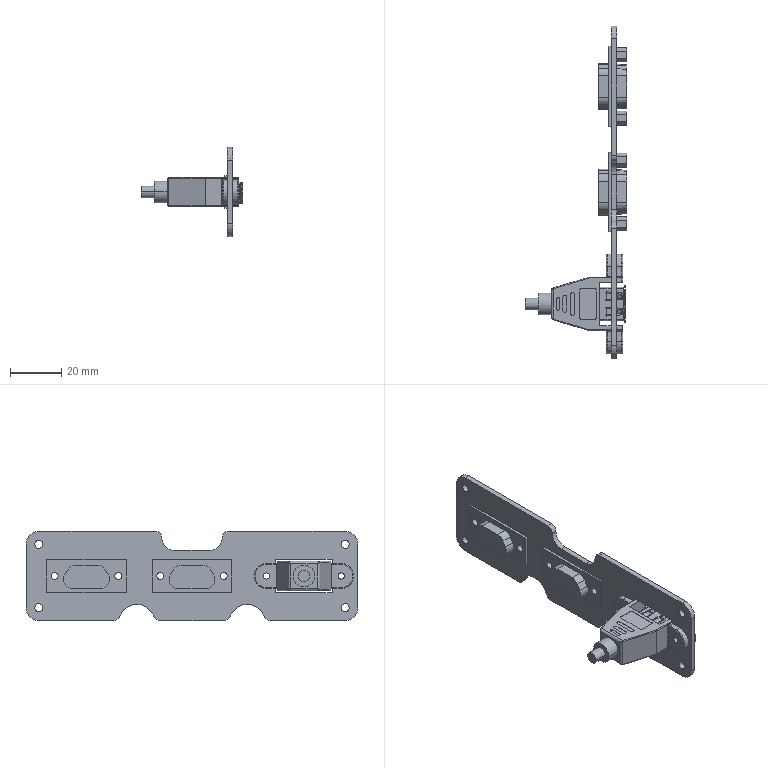Part | NX | features BREP 8 | 9 solids | 1294 faces | box 39.87 x 130 x 35 mm | volume 15905 mm3 | plane 745 | cylinder 433 | spline 50 | cone 46 | torus 14 | sphere 6 | commonest cylinder face diameters 0.6 x80 1 x68 0.4 x59 0.3 x24 1.2 x15 0.5 x12